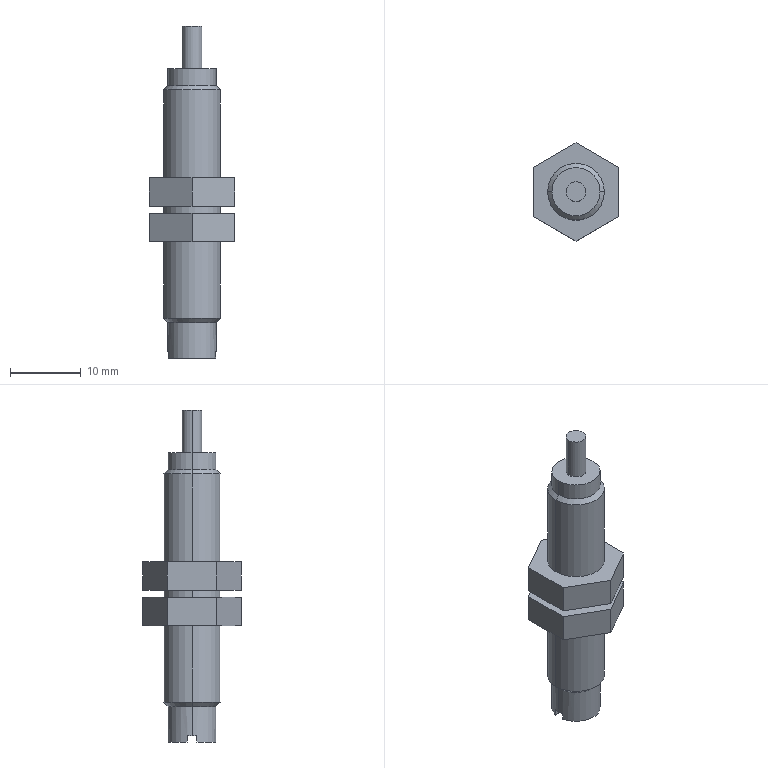Part | STEP file | Bag feed mounting electronic clip RB0806Z Z-axis | 1 solid | 39 faces | box 12 x 13.856 x 46.8 mm | volume 2563 mm3 | plane 23 | cylinder 12 | cone 4 | commonest cylinder face diameters 8 x6 6.8 x4 2.8 x2